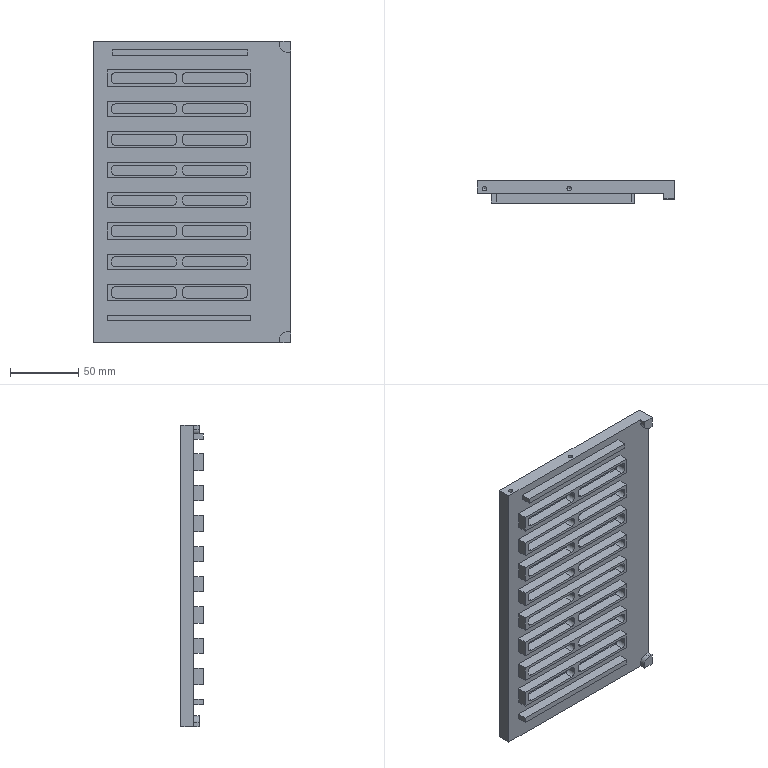NC program | NX | posted with a generic post | part box 144.5 x 16.5 x 221 mm
Lines 7394 to 8751 of 8751:
(FLOOR_WALL_1 , TOOL : D12-36-D12-120-3T-FINISH)
N14774 T20 M6
N14776 G53
N14778 G17 G0 G90 X1.505 Y-3.04 B0. C0. S4000 M3
N14780 G43 Z20. H20
N14782 Z-3.5
N14784 G94 G1 X2.265 Y-2.658 Z-3.545 F1000.
N14786 X6.037 Y-1.044 Z-3.76
N14788 X7.907 Y-0.376 Z-3.864
N14790 X6.484 Y0.28 Z-3.946
N14792 X3.712 Y1.744 Z-4.11
N14794 X2.368 Y2.55 Z-4.192
N14796 X-2.368 Z-4.44
N14798 X-3.962 Y1.594 Z-4.538
N14800 X-6.218 Y0.402 Z-4.672
N14802 X-7.907 Y-0.376 Z-4.769
N14804 X-6.037 Y-1.044 Z-4.873
N14806 X-2.265 Y-2.658 Z-5.088
N14808 X-0.491 Y-3.55 Z-5.192
N14810 X0.491 Z-5.244
N14812 X2.265 Y-2.658 Z-5.348
N14814 X6.037 Y-1.044 Z-5.563
N14816 X7.907 Y-0.376 Z-5.667
N14818 X6.484 Y0.28 Z-5.749
N14820 X3.712 Y1.744 Z-5.913
N14822 X2.368 Y2.55 Z-5.995
N14824 X-2.368 Z-6.244
N14826 X-3.962 Y1.594 Z-6.341
N14828 X-6.218 Y0.402 Z-6.475
N14830 X-7.907 Y-0.376 Z-6.572
N14832 X-6.037 Y-1.044 Z-6.676
N14834 X-2.265 Y-2.658 Z-6.891
N14836 X-0.491 Y-3.55 Z-6.995
N14838 X0.491 Z-7.047
N14840 X2.265 Y-2.658 Z-7.151
N14842 X6.037 Y-1.044 Z-7.366
N14844 X7.907 Y-0.376 Z-7.47
N14846 G2 X2.368 Y2.55 R57.6
N14848 G1 X-2.368
N14850 G2 X-7.907 Y-0.376 R57.6
N14852 G1 X-15.608 Y-0.596
N14854 X-7.907 Y-0.376
N14856 G2 X-0.491 Y-3.55 R65.7
N14858 G1 X0.491
N14860 G2 X7.907 Y-0.376 R65.7
N14862 G1 X15.608 Y-0.596
N14864 X7.907 Y-0.376
N14866 X29.55 Y4.006
N14868 G2 X5.158 Y12.15 R48.
N14870 G1 X-5.158
N14872 G2 X-43.194 Y5.267 R48.
N14874 G1 X-46.984 Y10.041
N14876 X-43.194 Y5.267
N14878 G2 X-44.576 Y-6.487 R48.
N14880 G1 X-49.193 Y-11.142
N14882 X-44.576 Y-6.487
N14884 G2 X-15.485 Y-8.06 R48.
N14886 X-2.863 Y-13.15 R56.1
N14888 G1 X2.863
N14890 G2 X15.485 Y-8.06 R56.1
N14892 X44.576 Y-6.487 R48.
N14894 G1 X49.193 Y-11.142
N14896 X44.576 Y-6.487
N14898 G2 X43.194 Y5.267 R48.
N14900 G1 X46.984 Y10.041
N14902 X43.194 Y5.267
N14904 G2 X29.55 Y4.006 R48.
N14906 G1 X8.274 Y21.75
N14908 X-8.274
N14910 G2 X-55.726 Y21.75 R38.4
N14912 G1 X-56.253
N14914 X-61.301 Y25.217
N14916 X-56.253 Y21.75
N14918 G2 X-55.46 Y19.009 R46.5
N14920 X-55.46 Y-9.109 R38.4
N14922 X-61. Y-22.086 R46.5
N14924 G1 Y-22.75
N14926 X-59.536
N14928 G2 X-46.559 Y-17.21 R46.5
N14930 X-18.441 Y-17.21 R38.4
N14932 X-5.464 Y-22.75 R46.5
N14934 G1 X5.464
N14936 G2 X18.441 Y-17.21 R46.5
N14938 X46.559 Y-17.21 R38.4
N14940 X59.536 Y-22.75 R46.5
N14942 G1 X61.
N14944 Y-22.086
N14946 G2 X55.46 Y-9.109 R46.5
N14948 X55.46 Y19.009 R38.4
N14950 X56.253 Y21.75 R46.5
N14952 G1 X61.301 Y25.217
N14954 X56.253 Y21.75
N14956 X55.726
N14958 G2 X8.274 Y21.75 R38.4
N14960 G1 X48.124 Y28.08
N14962 G2 X13.148 Y30.171 R28.8
N14964 X10.953 Y31.35 R36.9
N14966 G1 X-10.953
N14968 G2 X-13.148 Y30.171 R36.9
N14970 X-50.852 Y30.171 R28.8
N14972 X-53.047 Y31.35 R36.9
N14974 G1 X-70.6
N14976 Y29.074
N14978 G2 X-64.613 Y16.038 R36.9
N14980 X-64.613 Y-6.138 R28.8
N14982 X-70.6 Y-19.174 R36.9
N14984 G1 Y-32.35
N14986 X-56.624
N14988 G2 X-43.588 Y-26.363 R36.9
N14990 X-21.412 Y-26.363 R28.8
N14992 X-8.376 Y-32.35 R36.9
N14994 G1 X8.376
N14996 G2 X21.412 Y-26.363 R36.9
N14998 X43.588 Y-26.363 R28.8
N15000 X56.624 Y-32.35 R36.9
N15002 G1 X70.6
N15004 Y-19.174
N15006 G2 X64.613 Y-6.138 R36.9
N15008 X64.613 Y16.038 R28.8
N15010 X70.6 Y29.074 R36.9
N15012 G1 Y31.35
N15014 X53.047
N15016 G2 X50.852 Y30.171 R36.9
N15018 X48.124 Y28.08 R28.8
N15020 G1 X45.451 Y38.243
N15022 G2 X18.549 Y38.243 R19.2
N15024 X13.752 Y40.95 R27.3
N15026 G1 X-13.752
N15028 G2 X-18.549 Y38.243 R27.3
N15030 X-45.451 Y38.243 R19.2
N15032 X-50.248 Y40.95 R27.3
N15034 G1 X-77.252
N15036 G2 X-80.2 Y39.137 R27.3
N15038 G1 Y25.704
N15040 G2 X-73.776 Y13.03 R27.3
N15042 X-73.776 Y-3.13 R19.2
N15044 X-80.2 Y-15.804 R27.3
N15046 G1 Y-41.131
N15048 G2 X-79.246 Y-41.95 R27.3
N15050 G1 X-53.254
N15052 G2 X-40.58 Y-35.526 R27.3
N15054 X-24.42 Y-35.526 R19.2
N15056 X-11.746 Y-41.95 R27.3
N15058 G1 X11.746
N15060 G2 X24.42 Y-35.526 R27.3
N15062 X40.58 Y-35.526 R19.2
N15064 X53.254 Y-41.95 R27.3
N15066 G1 X79.246
N15068 G2 X80.2 Y-41.131 R27.3
N15070 G1 Y-15.804
N15072 G2 X73.776 Y-3.13 R27.3
N15074 X73.776 Y13.03 R19.2
N15076 X80.2 Y25.704 R27.3
N15078 G1 Y39.137
N15080 G2 X77.252 Y40.95 R27.3
N15082 G1 X50.248
N15084 G2 X45.451 Y38.243 R27.3
N15086 G1 X38.665 Y45.034
N15088 G2 X24.186 Y46.367 R9.6
N15090 X17.171 Y50.55 R17.7
N15092 G1 X-17.171
N15094 G2 X-24.186 Y46.367 R17.7
N15096 X-39.814 Y46.367 R9.6
N15098 X-46.829 Y50.55 R17.7
N15100 G1 X-80.671
N15102 G2 X-89.8 Y45.842 R17.7
N15104 G1 Y21.55
N15106 G2 X-82.971 Y9.905 R17.7
N15108 X-82.971 Y-0.005 R9.6
N15110 X-89.8 Y-11.65 R17.7
N15112 G1 Y-46.313
N15114 G2 X-83.4 Y-51.55 R17.7
N15116 G1 X-49.1
N15118 G2 X-37.455 Y-44.721 R17.7
N15120 X-27.545 Y-44.721 R9.6
N15122 X-15.9 Y-51.55 R17.7
N15124 G1 X15.9
N15126 G2 X27.545 Y-44.721 R17.7
N15128 X37.455 Y-44.721 R9.6
N15130 X49.1 Y-51.55 R17.7
N15132 G1 X83.4
N15134 G2 X89.8 Y-46.313 R17.7
N15136 G1 Y-11.65
N15138 G2 X82.971 Y-0.005 R17.7
N15140 X82.971 Y9.905 R9.6
N15142 X89.8 Y21.55 R17.7
N15144 G1 Y45.842
N15146 G2 X80.671 Y50.55 R17.7
N15148 G1 X46.829
N15150 G2 X39.814 Y46.367 R17.7
N15152 X38.665 Y45.034 R9.6
N15154 G1 X32. Y51.943
N15156 X29.873 Y55.15
N15158 X29.5
N15160 G2 X22.017 Y60.15 R8.1
N15162 G1 X-22.017
N15164 G2 X-29.5 Y55.15 R8.1
N15166 G1 X-29.873
N15168 X-32. Y51.943
N15170 X-34.127 Y55.15
N15172 X-34.5
N15174 G2 X-41.983 Y60.15 R8.1
N15176 G1 X-85.517
N15178 G2 X-93. Y55.15 R8.1
N15180 G1 X-99.4
N15182 Y15.475
N15184 G2 X-92.4 Y7.45 R8.1
N15186 G1 Y5.75
N15188 X-91.193 Y4.95
N15190 X-92.4 Y4.15
N15192 Y2.45
N15194 G2 X-99.4 Y-5.575 R8.1
N15196 G1 Y-54.15
N15198 X-97.5
N15200 G2 X-89.475 Y-61.15 R8.1
N15202 G1 X-43.025
N15204 G2 X-35. Y-54.15 R8.1
N15206 G1 X-33.3
N15208 X-32.5 Y-52.943
N15210 X-31.7 Y-54.15
N15212 X-30.
N15214 G2 X-21.975 Y-61.15 R8.1
N15216 G1 X21.975
N15218 G2 X30. Y-54.15 R8.1
N15220 G1 X31.7
N15222 X32.5 Y-52.943
N15224 X33.3 Y-54.15
N15226 X35.
N15228 G2 X43.025 Y-61.15 R8.1
N15230 G1 X89.475
N15232 G2 X97.5 Y-54.15 R8.1
N15234 G1 X99.4
N15236 Y-5.575
N15238 G2 X92.4 Y2.45 R8.1
N15240 G1 Y4.15
N15242 X91.193 Y4.95
N15244 X92.4 Y5.75
N15246 Y7.45
N15248 G2 X99.4 Y15.475 R8.1
N15250 G1 Y55.15
N15252 X93.
N15254 G2 X85.517 Y60.15 R8.1
N15256 G1 X41.983
N15258 G2 X34.5 Y55.15 R8.1
N15260 G1 X34.127
N15262 X32. Y51.943
N15264 X31.447 Y52.777
N15266 G2 X31.868 Y54.856 R1.5
N15268 G1 Z-4.47
N15270 G0 Z20.
N15272 M5
(PLANAR_MILL , TOOL : D8-25-D8-60-3T-FINISH)
N15274 T04 M6
N15276 G53
N15278 G17 G0 G90 X-119.5 Y76.35 B0. C0. S4000 M3
N15280 G43 Z20. H4
N15282 Z-13.
N15284 G94 G1 Z-15. F1000.
N15286 X-110.5
N15288 X110.5
N15290 X119.5
N15292 Z-13.
N15294 G0 Z20.
N15296 Y-76.35
N15298 Z-13.
N15300 G1 Z-15.
N15302 X110.5
N15304 X-110.5
N15306 X-119.5
N15308 Z-13.
N15310 G0 Z20.
(PLANAR_MILL_COPY , TOOL : D8-25-D8-60-3T-FINISH)
N15312 X-114.53 Y-81.25
N15314 Z-13.
N15316 G1 Z-15.
N15318 Y-72.25
N15320 Y72.25
N15322 Y81.25
N15324 Z-13.
N15326 G0 Z20.
N15328 X114.53
N15330 Z-13.
N15332 G1 Z-15.
N15334 Y72.25
N15336 Y-72.25
N15338 Y-81.25
N15340 Z-13.
N15342 G0 Z20.
N15344 M5
(FLOOR_WALL_1_COPY , TOOL : D5-15-D6-50-3T-FINISH)
N15346 T05 M6
N15348 G53
N15350 G17 G0 G90 X0.301 Y-1.523 B0. C0. S4000 M3
N15352 G43 Z20. H5
N15354 Z-6.5
N15356 G94 G1 X1.849 Y-0.757 Z-6.59 F1000.
N15358 X2.741 Y-0.357 Z-6.642
N15360 X4.608 Y0.4 Z-6.747
N15362 X4.296 Y0.523 Z-6.765
N15364 X3.985 Y0.65 Z-6.782
N15366 X-3.985 Z-7.2
N15368 X-4.296 Y0.523 Z-7.218
N15370 X-4.608 Y0.4 Z-7.235
N15372 X-2.741 Y-0.357 Z-7.341
N15374 X-1.849 Y-0.757 Z-7.392
N15376 X-0.043 Y-1.65 Z-7.498
N15378 X0. Z-7.5
N15380 X0.043
N15382 G2 X4.608 Y0.4 R67.6
N15384 G1 X7.216 Y0.41
N15386 X4.608 Y0.4
N15388 G2 X3.985 Y0.65 R67.6
N15390 G1 X-3.985
N15392 G2 X-4.608 Y0.4 R67.6
N15394 G1 X-7.216 Y0.41
N15396 X-4.608 Y0.4
N15398 G2 X-0.043 Y-1.65 R67.6
N15400 G1 X0.
N15402 Y-5.15
N15404 X0.873
N15406 G2 X16.666 Y0.448 R64.1
N15408 G1 X19.102 Y1.013
N15410 G3 X23.118 Y0.474 R63.1
N15412 X19.106 Y-0.097 R63.1
N15414 X19.102 Y1.013 R2.5
N15416 G1 X16.666 Y0.448
N15418 G2 X4.681 Y4.15 R64.1
N15420 G1 X-4.681
N15422 G2 X-16.666 Y0.448 R64.1
N15424 G1 X-19.106 Y-0.097
N15426 G3 X-23.118 Y0.474 R63.1
N15428 X-19.102 Y1.013 R63.1
N15430 X-19.106 Y-0.097 R2.5
N15432 G1 X-16.666 Y0.448
N15434 G2 X-0.873 Y-5.15 R64.1
N15436 G1 X0.
N15438 Y-8.65
N15440 X1.726
N15442 G2 X30. Y-1.65 R60.6
N15444 G1 X35.
N15446 G2 X40.054 Y-1.861 R60.6
N15448 X39.9 Y2.45 R60.6
N15450 G1 Y2.891
N15452 G2 X34.5 Y2.65 R60.6
N15454 G1 X29.5
N15456 G2 X5.396 Y7.65 R60.6
N15458 G1 X-5.396
N15460 G2 X-29.5 Y2.65 R60.6
N15462 G1 X-34.5
N15464 G2 X-39.9 Y2.891 R60.6
N15466 G1 Y2.45
N15468 G2 X-40.054 Y-1.861 R60.6
N15470 X-35. Y-1.65 R60.6
N15472 G1 X-30.
N15474 G2 X-1.726 Y-8.65 R60.6
N15476 G1 X0.
N15478 Y-12.15
N15480 X2.607
N15482 G2 X30. Y-5.15 R57.1
N15484 G1 X35.
N15486 G2 X44.009 Y-5.865 R57.1
N15488 X43.4 Y2.45 R57.1
N15490 G1 Y6.848
N15492 G2 X34.5 Y6.15 R57.1
N15494 G1 X29.5
N15496 G2 X6.133 Y11.15 R57.1
N15498 G1 X-6.133
N15500 G2 X-29.5 Y6.15 R57.1
N15502 G1 X-34.5
N15504 G2 X-43.4 Y6.848 R57.1
N15506 G1 Y2.45
N15508 G2 X-44.009 Y-5.865 R57.1
N15510 X-35. Y-5.15 R57.1
N15512 G1 X-30.
N15514 G2 X-2.607 Y-12.15 R57.1
N15516 G1 X0.
N15518 Y-15.65
N15520 X3.516
N15522 G2 X30. Y-8.65 R53.6
N15524 G1 X35.
N15526 G2 X48.455 Y-10.366 R53.6
N15528 X46.9 Y2.45 R53.6
N15530 G1 Y7.45
N15532 G2 X47.027 Y11.134 R53.6
N15534 X34.5 Y9.65 R53.6
N15536 G1 X29.5
N15538 G2 X6.895 Y14.65 R53.6
N15540 G1 X-6.895
N15542 G2 X-29.5 Y9.65 R53.6
N15544 G1 X-34.5
N15546 G2 X-47.027 Y11.134 R53.6
N15548 X-46.9 Y7.45 R53.6
N15550 G1 Y2.45
N15552 G2 X-48.455 Y-10.366 R53.6
N15554 X-35. Y-8.65 R53.6
N15556 G1 X-30.
N15558 G2 X-3.516 Y-15.65 R53.6
N15560 G1 X0.
N15562 Y-19.15
N15564 X4.458
N15566 G2 X30. Y-12.15 R50.1
N15568 G1 X35.
N15570 G2 X53.855 Y-15.834 R50.1
N15572 G1 X55.657 Y-17.657
N15574 X53.855 Y-15.834
N15576 G2 X50.4 Y2.45 R50.1
N15578 G1 Y7.45
N15580 G2 X51.134 Y15.992 R50.1
N15582 X34.5 Y13.15 R50.1
N15584 G1 X29.5
N15586 G2 X7.683 Y18.15 R50.1
N15588 G1 X-7.683
N15590 G2 X-29.5 Y13.15 R50.1
N15592 G1 X-34.5
N15594 G2 X-51.134 Y15.992 R50.1
N15596 X-50.4 Y7.45 R50.1
N15598 G1 Y2.45
N15600 G2 X-53.855 Y-15.834 R50.1
N15602 G1 X-55.657 Y-17.657
N15604 X-53.855 Y-15.834
N15606 G2 X-35. Y-12.15 R50.1
N15608 G1 X-30.
N15610 G2 X-4.458 Y-19.15 R50.1
N15612 G1 X0.
N15614 Y-22.65
N15616 X5.436
N15618 G2 X30. Y-15.65 R46.6
N15620 G1 X35.
N15622 G2 X59.564 Y-22.65 R46.6
N15624 G1 X60.9
N15626 Y-22.114
N15628 G2 X53.9 Y2.45 R46.6
N15630 G1 Y7.45
N15632 G2 X56.116 Y21.65 R46.6
N15634 G1 X55.5
N15636 G2 X34.5 Y16.65 R46.6
N15638 G1 X29.5
N15640 G2 X8.5 Y21.65 R46.6
N15642 G1 X-8.5
N15644 G2 X-29.5 Y16.65 R46.6
N15646 G1 X-34.5
N15648 G2 X-55.5 Y21.65 R46.6
N15650 G1 X-56.116
N15652 G2 X-53.9 Y7.45 R46.6
N15654 G1 Y2.45
N15656 G2 X-60.9 Y-22.114 R46.6
N15658 G1 Y-22.65
N15660 X-59.564
N15662 G2 X-35. Y-15.65 R46.6
N15664 G1 X-30.
N15666 G2 X-5.436 Y-22.65 R46.6
N15668 G1 X0.
N15670 Y-26.15
N15672 X6.454
N15674 G2 X30. Y-19.15 R43.1
N15676 G1 X35.
N15678 G2 X58.546 Y-26.15 R43.1
N15680 G1 X64.4
N15682 Y-21.096
N15684 G2 X57.4 Y2.45 R43.1
N15686 G1 Y7.45
N15688 G2 X61.202 Y25.15 R43.1
N15690 G1 X54.649
N15692 G2 X34.5 Y20.15 R43.1
N15694 G1 X29.5
N15696 G2 X9.351 Y25.15 R43.1
N15698 G1 X-9.351
N15700 G2 X-29.5 Y20.15 R43.1
N15702 G1 X-34.5
N15704 G2 X-54.649 Y25.15 R43.1
N15706 G1 X-61.202
N15708 G2 X-57.4 Y7.45 R43.1
N15710 G1 Y2.45
N15712 G2 X-64.4 Y-21.096 R43.1
N15714 G1 Y-26.15
N15716 X-58.546
N15718 G2 X-35. Y-19.15 R43.1
N15720 G1 X-30.
N15722 G2 X-6.454 Y-26.15 R43.1
N15724 G1 X0.
N15726 Y-29.65
N15728 X7.519
N15730 G2 X30. Y-22.65 R39.6
N15732 G1 X35.
N15734 G2 X57.481 Y-29.65 R39.6
N15736 G1 X67.9
N15738 Y-20.031
N15740 G2 X60.9 Y2.45 R39.6
N15742 G1 Y7.45
N15744 G2 X67.053 Y28.65 R39.6
N15746 G1 X53.761
N15748 G2 X34.5 Y23.65 R39.6
N15750 G1 X29.5
N15752 G2 X10.239 Y28.65 R39.6
N15754 G1 X-10.239
N15756 G2 X-29.5 Y23.65 R39.6
N15758 G1 X-34.5
N15760 G2 X-53.761 Y28.65 R39.6
N15762 G1 X-67.053
N15764 G2 X-60.9 Y7.45 R39.6
N15766 G1 Y2.45
N15768 G2 X-67.9 Y-20.031 R39.6
N15770 G1 Y-29.65
N15772 X-57.481
N15774 G2 X-35. Y-22.65 R39.6
N15776 G1 X-30.
N15778 G2 X-7.519 Y-29.65 R39.6
N15780 G1 X0.
N15782 Y-33.15
N15784 X8.636
N15786 G2 X30. Y-26.15 R36.1
N15788 G1 X35.
N15790 G2 X56.364 Y-33.15 R36.1
N15792 G1 X71.4
N15794 Y-18.914
N15796 G2 X64.4 Y2.45 R36.1
N15798 G1 Y7.45
N15800 G2 X71.4 Y28.814 R36.1
N15802 G1 Y32.15
N15804 X52.83
N15806 G2 X34.5 Y27.15 R36.1
N15808 G1 X29.5
N15810 G2 X11.17 Y32.15 R36.1
N15812 G1 X-11.17
N15814 G2 X-29.5 Y27.15 R36.1
N15816 G1 X-34.5
N15818 G2 X-52.83 Y32.15 R36.1
N15820 G1 X-71.4
N15822 Y28.814
N15824 G2 X-64.4 Y7.45 R36.1
N15826 G1 Y2.45
N15828 G2 X-71.4 Y-18.914 R36.1
N15830 G1 Y-33.15
N15832 X-56.364
N15834 G2 X-35. Y-26.15 R36.1
N15836 G1 X-30.
N15838 G2 X-8.636 Y-33.15 R36.1
N15840 G1 X0.
N15842 Y-36.65
N15844 X9.816
N15846 G2 X30. Y-29.65 R32.6
N15848 G1 X35.
N15850 G2 X55.184 Y-36.65 R32.6
N15852 G1 X74.9
N15854 Y-17.734
N15856 G2 X67.9 Y2.45 R32.6
N15858 G1 Y7.45
N15860 G2 X74.9 Y27.634 R32.6
N15862 G1 Y35.65
N15864 X51.849
N15866 G2 X34.5 Y30.65 R32.6
N15868 G1 X29.5
N15870 G2 X12.151 Y35.65 R32.6
N15872 G1 X-12.151
N15874 G2 X-29.5 Y30.65 R32.6
N15876 G1 X-34.5
N15878 G2 X-51.849 Y35.65 R32.6
N15880 G1 X-74.9
N15882 Y27.634
N15884 G2 X-67.9 Y7.45 R32.6
N15886 G1 Y2.45
N15888 G2 X-74.9 Y-17.734 R32.6
N15890 G1 Y-36.65
N15892 X-55.184
N15894 G2 X-35. Y-29.65 R32.6
N15896 G1 X-30.
N15898 G2 X-9.816 Y-36.65 R32.6
N15900 G1 X0.
N15902 Y-40.15
N15904 X11.069
N15906 G2 X30. Y-33.15 R29.1
N15908 G1 X35.
N15910 G2 X53.931 Y-40.15 R29.1
N15912 G1 X78.4
N15914 Y-16.481
N15916 G2 X71.4 Y2.45 R29.1
N15918 G1 Y7.45
N15920 G2 X78.4 Y26.381 R29.1
N15922 G1 Y38.078
N15924 G2 X76.69 Y39.15 R29.1
N15926 G1 X50.81
N15928 G2 X34.5 Y34.15 R29.1
N15930 G1 X29.5
N15932 G2 X13.19 Y39.15 R29.1
N15934 G1 X-13.19
N15936 G2 X-29.5 Y34.15 R29.1
N15938 G1 X-34.5
N15940 G2 X-50.81 Y39.15 R29.1
N15942 G1 X-76.69
N15944 G2 X-78.4 Y38.078 R29.1
N15946 G1 Y26.381
N15948 G2 X-71.4 Y7.45 R29.1
N15950 G1 Y2.45
N15952 G2 X-78.4 Y-16.481 R29.1
N15954 G1 Y-40.15
N15956 X-53.931
N15958 G2 X-35. Y-33.15 R29.1
N15960 G1 X-30.
N15962 G2 X-11.069 Y-40.15 R29.1
N15964 G1 X0.
N15966 Y-43.65
N15968 X12.41
N15970 G2 X30. Y-36.65 R25.6
N15972 G1 X35.
N15974 G2 X52.59 Y-43.65 R25.6
N15976 G1 X79.91
N15978 G2 X81.9 Y-41.952 R25.6
N15980 G1 Y-15.14
N15982 G2 X74.9 Y2.45 R25.6
N15984 G1 Y7.45
N15986 G2 X81.9 Y25.04 R25.6
N15988 G1 Y40.182
N15990 G2 X77.801 Y42.65 R25.6
N15992 G1 X49.699
N15994 G2 X34.5 Y37.65 R25.6
N15996 G1 X29.5
N15998 G2 X14.301 Y42.65 R25.6
N16000 G1 X-14.301
N16002 G2 X-29.5 Y37.65 R25.6
N16004 G1 X-34.5
N16006 G2 X-49.699 Y42.65 R25.6
N16008 G1 X-77.801
N16010 G2 X-81.9 Y40.182 R25.6
N16012 G1 Y25.04
N16014 G2 X-74.9 Y7.45 R25.6
N16016 G1 Y2.45
N16018 G2 X-81.9 Y-15.14 R25.6
N16020 G1 Y-41.952
N16022 G2 X-79.91 Y-43.65 R25.6
N16024 G1 X-52.59
N16026 G2 X-35. Y-36.65 R25.6
N16028 G1 X-30.
N16030 G2 X-12.41 Y-43.65 R25.6
N16032 G1 X0.
N16034 Y-47.15
N16036 X13.863
N16038 G2 X30. Y-40.15 R22.1
N16040 G1 X35.
N16042 G2 X51.137 Y-47.15 R22.1
N16044 G1 X81.363
N16046 G2 X85.4 Y-43.757 R22.1
N16048 G1 Y-13.687
N16050 G2 X78.4 Y2.45 R22.1
N16052 G1 Y7.45
N16054 G2 X85.4 Y23.587 R22.1
N16056 G1 Y42.498
N16058 G2 X79. Y46.15 R22.1
N16060 G1 X48.5
N16062 G2 X34.5 Y41.15 R22.1
N16064 G1 X29.5
N16066 G2 X15.5 Y46.15 R22.1
N16068 G1 X-15.5
N16070 G2 X-29.5 Y41.15 R22.1
N16072 G1 X-34.5
N16074 G2 X-48.5 Y46.15 R22.1
N16076 G1 X-79.
N16078 G2 X-85.4 Y42.498 R22.1
N16080 G1 Y23.587
N16082 G2 X-78.4 Y7.45 R22.1
N16084 G1 Y2.45
N16086 G2 X-85.4 Y-13.687 R22.1
N16088 G1 Y-43.757
N16090 G2 X-81.363 Y-47.15 R22.1
N16092 G1 X-51.137
N16094 G2 X-35. Y-40.15 R22.1
N16096 G1 X-30.
N16098 G2 X-13.863 Y-47.15 R22.1
N16100 G1 X0.
N16102 Y-50.65
N16104 X15.46
N16106 G2 X30. Y-43.65 R18.6
N16108 G1 X35.
N16110 G2 X49.54 Y-50.65 R18.6
N16112 G1 X82.96
N16114 G2 X88.9 Y-45.758 R18.6
N16116 G1 Y-12.09
N16118 G2 X81.9 Y2.45 R18.6
N16120 G1 Y7.45
N16122 G2 X88.9 Y21.99 R18.6
N16124 G1 Y45.108
N16126 G2 X80.311 Y49.65 R18.6
N16128 G1 X47.189
N16130 G2 X34.5 Y44.65 R18.6
N16132 G1 X29.5
N16134 G2 X16.811 Y49.65 R18.6
N16136 G1 X-16.811
N16138 G2 X-29.5 Y44.65 R18.6
N16140 G1 X-34.5
N16142 G2 X-47.189 Y49.65 R18.6
N16144 G1 X-80.311
N16146 G2 X-88.9 Y45.108 R18.6
N16148 G1 Y21.99
N16150 G2 X-81.9 Y7.45 R18.6
N16152 G1 Y2.45
N16154 G2 X-88.9 Y-12.09 R18.6
N16156 G1 Y-45.758
N16158 G2 X-82.96 Y-50.65 R18.6
N16160 G1 X-49.54
N16162 G2 X-35. Y-43.65 R18.6
N16164 G1 X-30.
N16166 G2 X-15.46 Y-50.65 R18.6
N16168 G1 X0.
N16170 Y-54.15
N16172 X17.256
N16174 G2 X30. Y-47.15 R15.1
N16176 G1 X35.
N16178 G2 X47.744 Y-54.15 R15.1
N16180 G1 X84.756
N16182 G2 X92.4 Y-48.037 R15.1
N16184 G1 Y-10.294
N16186 G2 X85.4 Y2.45 R15.1
N16188 G1 Y7.45
N16190 G2 X92.4 Y20.194 R15.1
N16192 G1 Y48.162
N16194 G2 X81.775 Y53.15 R15.1
N16196 G1 X45.725
N16198 G2 X34.5 Y48.15 R15.1
N16200 G1 X29.5
N16202 G2 X18.275 Y53.15 R15.1
N16204 G1 X-18.275
N16206 G2 X-29.5 Y48.15 R15.1
N16208 G1 X-34.5
N16210 G2 X-45.725 Y53.15 R15.1
N16212 G1 X-81.775
N16214 G2 X-92.4 Y48.162 R15.1
N16216 G1 Y20.194
N16218 G2 X-85.4 Y7.45 R15.1
N16220 G1 Y2.45
N16222 G2 X-92.4 Y-10.294 R15.1
N16224 G1 Y-48.037
N16226 G2 X-84.756 Y-54.15 R15.1
N16228 G1 X-47.744
N16230 G2 X-35. Y-47.15 R15.1
N16232 G1 X-30.
N16234 G2 X-17.256 Y-54.15 R15.1
N16236 G1 X0.
N16238 Y-57.65
N16240 X19.351
N16242 G2 X30. Y-50.65 R11.6
N16244 G1 X35.
N16246 G2 X45.649 Y-57.65 R11.6
N16248 G1 X86.851
N16250 G2 X95.9 Y-50.761 R11.6
N16252 G1 Y-8.199
N16254 G2 X88.9 Y2.45 R11.6
N16256 G1 Y7.45
N16258 G2 X95.9 Y18.099 R11.6
N16260 G1 Y51.65
N16262 X93.
N16264 G2 X83.461 Y56.65 R11.6
N16266 G1 X44.039
N16268 G2 X34.5 Y51.65 R11.6
N16270 G1 X29.5
N16272 G2 X19.961 Y56.65 R11.6
N16274 G1 X-19.961
N16276 G2 X-29.5 Y51.65 R11.6
N16278 G1 X-34.5
N16280 G2 X-44.039 Y56.65 R11.6
N16282 G1 X-83.461
N16284 G2 X-93. Y51.65 R11.6
N16286 G1 X-95.9
N16288 Y18.099
N16290 G2 X-88.9 Y7.45 R11.6
N16292 G1 Y2.45
N16294 G2 X-95.9 Y-8.199 R11.6
N16296 G1 Y-50.761
N16298 G2 X-86.851 Y-57.65 R11.6
N16300 G1 X-45.649
N16302 G2 X-35. Y-50.65 R11.6
N16304 G1 X-30.
N16306 G2 X-19.351 Y-57.65 R11.6
N16308 G1 X0.
N16310 Y-61.15
N16312 X21.975
N16314 G2 X30. Y-54.15 R8.1
N16316 G1 X35.
N16318 G2 X43.025 Y-61.15 R8.1
N16320 G1 X89.475
N16322 G2 X97.5 Y-54.15 R8.1
N16324 G1 X99.4
N16326 Y-5.575
N16328 G2 X92.4 Y2.45 R8.1
N16330 G1 Y7.45
N16332 G2 X99.4 Y15.475 R8.1
N16334 G1 Y55.15
N16336 X93.
N16338 G2 X85.517 Y60.15 R8.1
N16340 G1 X41.983
N16342 G2 X34.5 Y55.15 R8.1
N16344 G1 X29.5
N16346 G2 X22.017 Y60.15 R8.1
N16348 G1 X-22.017
N16350 G2 X-29.5 Y55.15 R8.1
N16352 G1 X-34.5
N16354 G2 X-41.983 Y60.15 R8.1
N16356 G1 X-85.517
N16358 G2 X-93. Y55.15 R8.1
N16360 G1 X-99.4
N16362 Y15.475
N16364 G2 X-92.4 Y7.45 R8.1
N16366 G1 Y2.45
N16368 G2 X-99.4 Y-5.575 R8.1
N16370 G1 Y-54.15
N16372 X-97.5
N16374 G2 X-89.475 Y-61.15 R8.1
N16376 G1 X-43.025
N16378 G2 X-35. Y-54.15 R8.1
N16380 G1 X-30.
N16382 G2 X-21.975 Y-61.15 R8.1
N16384 G1 X0.
N16386 Y-64.65
N16388 X24.975
N16390 G3 X25.387 Y-64.347 R0.42
N16392 G1 X25.4 Y-64.218
N16394 Y-62.25
N16396 G2 X30. Y-57.65 R4.6
N16398 G1 X35.
N16400 G2 X39.6 Y-62.25 R4.6
N16402 G1 X39.603 Y-64.291
N16404 G3 X40.032 Y-64.65 R0.418
N16406 G1 X92.475
N16408 X92.754 Y-64.558
N16410 X92.845 Y-64.505
N16412 X92.869 Y-64.402
N16414 X92.9 Y-64.218
N16416 Y-62.25
N16418 G2 X97.5 Y-57.65 R4.6
N16420 G1 X102.5
N16422 G3 X102.9 Y-57.25 R0.4
N16424 G1 Y-2.55
N16426 G3 X102.5 Y-2.15 R0.4
N16428 G1 X100.5
N16430 G2 X95.9 Y2.45 R4.6
N16432 G1 Y7.45
N16434 G2 X100.5 Y12.05 R4.6
N16436 G1 X102.5
N16438 G3 X102.9 Y12.45 R0.4
N16440 G1 Y58.25
N16442 G3 X102.5 Y58.65 R0.4
N16444 G1 X93.
N16446 G2 X88.4 Y63.25 R4.6
N16448 G3 X88. Y63.65 R0.4
N16450 G1 X39.5
N16452 G3 X39.1 Y63.25 R0.4
N16454 G2 X34.5 Y58.65 R4.6
N16456 G1 X29.5
N16458 G2 X24.9 Y63.25 R4.6
N16460 G3 X24.5 Y63.65 R0.4
N16462 G1 X-24.5
N16464 G3 X-24.9 Y63.25 R0.4
N16466 G2 X-29.5 Y58.65 R4.6
N16468 G1 X-34.5
N16470 G2 X-39.1 Y63.25 R4.6
N16472 G3 X-39.5 Y63.65 R0.4
N16474 G1 X-88.
N16476 G3 X-88.4 Y63.25 R0.4
N16478 G2 X-93. Y58.65 R4.6
N16480 G1 X-102.5
N16482 G3 X-102.9 Y58.25 R0.4
N16484 G1 Y12.45
N16486 G3 X-102.5 Y12.05 R0.4
N16488 G1 X-100.5
N16490 G2 X-95.9 Y7.45 R4.6
N16492 G1 Y2.45
N16494 G2 X-100.5 Y-2.15 R4.6
N16496 G1 X-102.5
N16498 G3 X-102.9 Y-2.55 R0.4
N16500 G1 Y-57.25
N16502 G3 X-102.5 Y-57.65 R0.4
N16504 G1 X-97.5
N16506 G2 X-92.9 Y-62.25 R4.6
N16508 G1 X-92.897 Y-64.291
N16510 G3 X-92.688 Y-64.602 R0.399
N16512 G1 X-92.468 Y-64.65
N16514 X-40.025
N16516 G3 X-39.631 Y-64.402 R0.42
N16518 G1 X-39.575 Y-64.317
N16520 X-39.6 Y-64.218
N16522 Y-62.25
N16524 G2 X-35. Y-57.65 R4.6
N16526 G1 X-30.
N16528 G2 X-25.4 Y-62.25 R4.6
N16530 G1 X-25.399 Y-64.271
N16532 X-25.391 Y-64.33
N16534 G3 X-24.968 Y-64.65 R0.419
N16536 G1 X0.
N16538 X1.
N16540 G3 X2.25 Y-63.4 R1.25
N16542 G1 Z-4.5
N16544 G0 Z20.
(PLANAR_MILL_1 , TOOL : D5-15-D6-50-3T-FINISH)
N16546 X-100.5 Y56.72 S3500
N16548 Z-5.48
N16550 G1 Z-7.48 F800.
N16552 G3 X-102.5 Y58.72 R2.
N16554 X-102.97 Y58.25 R0.47
N16556 G1 Y12.45
N16558 G3 X-102.5 Y11.98 R0.47
N16560 G1 X-100.5
N16562 G2 X-95.97 Y7.45 R4.53
N16564 G1 Y2.45
N16566 G2 X-100.5 Y-2.08 R4.53
N16568 G1 X-102.5
N16570 G3 X-102.97 Y-2.55 R0.47
N16572 G1 Y-57.25
N16574 G3 X-102.5 Y-57.72 R0.47
N16576 G1 X-97.5
N16578 G2 X-92.97 Y-62.25 R4.53
N16580 G1 Y-64.25
N16582 G3 X-92.5 Y-64.72 R0.47
N16584 G1 X-40.
N16586 G3 X-39.53 Y-64.25 R0.47
N16588 G1 Y-62.25
N16590 G2 X-35. Y-57.72 R4.53
N16592 G1 X-30.
N16594 G2 X-25.47 Y-62.25 R4.53
N16596 G1 Y-64.25
N16598 G3 X-25. Y-64.72 R0.47
N16600 G1 X25.
N16602 G3 X25.47 Y-64.25 R0.47
N16604 G1 Y-62.25
N16606 G2 X30. Y-57.72 R4.53
N16608 G1 X35.
N16610 G2 X39.53 Y-62.25 R4.53
N16612 G1 Y-64.25
N16614 G3 X40. Y-64.72 R0.47
N16616 G1 X92.5
N16618 G3 X92.97 Y-64.25 R0.47
N16620 G1 Y-62.25
N16622 G2 X97.5 Y-57.72 R4.53
N16624 G1 X102.5
N16626 G3 X102.97 Y-57.25 R0.47
N16628 G1 Y-2.55
N16630 G3 X102.5 Y-2.08 R0.47
N16632 G1 X100.5
N16634 G2 X95.97 Y2.45 R4.53
N16636 G1 Y7.45
N16638 G2 X100.5 Y11.98 R4.53
N16640 G1 X102.5
N16642 G3 X102.97 Y12.45 R0.47
N16644 G1 Y58.25
N16646 G3 X102.5 Y58.72 R0.47
N16648 G1 X93.
N16650 G2 X88.47 Y63.25 R4.53
N16652 G3 X88. Y63.72 R0.47
N16654 G1 X39.5
N16656 G3 X39.03 Y63.25 R0.47
N16658 G2 X34.5 Y58.72 R4.53
N16660 G1 X29.5
N16662 G2 X24.97 Y63.25 R4.53
N16664 G3 X24.5 Y63.72 R0.47
N16666 G1 X-24.5
N16668 G3 X-24.97 Y63.25 R0.47
N16670 G2 X-29.5 Y58.72 R4.53
N16672 G1 X-34.5
N16674 G2 X-39.03 Y63.25 R4.53
N16676 G3 X-39.5 Y63.72 R0.47
N16678 G1 X-88.
N16680 G3 X-88.47 Y63.25 R0.47
N16682 G2 X-93. Y58.72 R4.53
N16684 G1 X-102.5
N16686 G3 X-100.5 Y56.72 R2.
N16688 X-102.5 Y58.72 R2.
N16690 X-102.97 Y58.25 R0.47
N16692 G1 Y12.45
N16694 G3 X-102.5 Y11.98 R0.47
N16696 G1 X-100.5
N16698 G2 X-95.97 Y7.45 R4.53
N16700 G1 Y2.45
N16702 G2 X-100.5 Y-2.08 R4.53
N16704 G1 X-102.5
N16706 G3 X-102.97 Y-2.55 R0.47
N16708 G1 Y-57.25
N16710 G3 X-102.5 Y-57.72 R0.47
N16712 G1 X-97.5
N16714 G2 X-92.97 Y-62.25 R4.53
N16716 G1 Y-64.25
N16718 G3 X-92.5 Y-64.72 R0.47
N16720 G1 X-40.
N16722 G3 X-39.53 Y-64.25 R0.47
N16724 G1 Y-62.25
N16726 G2 X-35. Y-57.72 R4.53
N16728 G1 X-30.
N16730 G2 X-25.47 Y-62.25 R4.53
N16732 G1 Y-64.25
N16734 G3 X-25. Y-64.72 R0.47
N16736 G1 X25.
N16738 G3 X25.47 Y-64.25 R0.47
N16740 G1 Y-62.25
N16742 G2 X30. Y-57.72 R4.53
N16744 G1 X35.
N16746 G2 X39.53 Y-62.25 R4.53
N16748 G1 Y-64.25
N16750 G3 X40. Y-64.72 R0.47
N16752 G1 X92.5
N16754 G3 X92.97 Y-64.25 R0.47
N16756 G1 Y-62.25
N16758 G2 X97.5 Y-57.72 R4.53
N16760 G1 X102.5
N16762 G3 X102.97 Y-57.25 R0.47
N16764 G1 Y-2.55
N16766 G3 X102.5 Y-2.08 R0.47
N16768 G1 X100.5
N16770 G2 X95.97 Y2.45 R4.53
N16772 G1 Y7.45
N16774 G2 X100.5 Y11.98 R4.53
N16776 G1 X102.5
N16778 G3 X102.97 Y12.45 R0.47
N16780 G1 Y58.25
N16782 G3 X102.5 Y58.72 R0.47
N16784 G1 X93.
N16786 G2 X88.47 Y63.25 R4.53
N16788 G3 X88. Y63.72 R0.47
N16790 G1 X39.5
N16792 G3 X39.03 Y63.25 R0.47
N16794 G2 X34.5 Y58.72 R4.53
N16796 G1 X29.5
N16798 G2 X24.97 Y63.25 R4.53
N16800 G3 X24.5 Y63.72 R0.47
N16802 G1 X-24.5
N16804 G3 X-24.97 Y63.25 R0.47
N16806 G2 X-29.5 Y58.72 R4.53
N16808 G1 X-34.5
N16810 G2 X-39.03 Y63.25 R4.53
N16812 G3 X-39.5 Y63.72 R0.47
N16814 G1 X-88.
N16816 G3 X-88.47 Y63.25 R0.47
N16818 G2 X-93. Y58.72 R4.53
N16820 G1 X-102.5
N16822 G3 X-100.5 Y56.72 R2.
N16824 G1 Z-5.48
N16826 G0 Z20.
N16828 M5
(PLANAR_MILL_1_COPY , TOOL : 倒角D6-90度)
N16830 T06 M6
N16832 G53
N16834 G17 G0 G90 X-100.5 Y57.75 B0. C0. S3500 M3
N16836 G43 Z20. H6
N16838 Z0.5
N16840 G94 G1 Z-1.5 F1000.
N16842 G3 X-102.5 Y59.75 R2.
N16844 X-104. Y58.25 R1.5
N16846 G1 Y12.45
N16848 G3 X-102.5 Y10.95 R1.5
N16850 G1 X-100.5
N16852 G2 X-97. Y7.45 R3.5
N16854 G1 Y2.45
N16856 G2 X-100.5 Y-1.05 R3.5
N16858 G1 X-102.5
N16860 G3 X-104. Y-2.55 R1.5
N16862 G1 Y-57.25
N16864 G3 X-102.5 Y-58.75 R1.5
N16866 G1 X-97.5
N16868 G2 X-94. Y-62.25 R3.5
N16870 G1 Y-64.25
N16872 G3 X-92.5 Y-65.75 R1.5
N16874 G1 X-40.
N16876 G3 X-38.5 Y-64.25 R1.5
N16878 G1 Y-62.25
N16880 G2 X-35. Y-58.75 R3.5
N16882 G1 X-30.
N16884 G2 X-26.5 Y-62.25 R3.5
N16886 G1 Y-64.25
N16888 G3 X-25. Y-65.75 R1.5
N16890 G1 X25.
N16892 G3 X26.5 Y-64.25 R1.5
N16894 G1 Y-62.25
N16896 G2 X30. Y-58.75 R3.5
N16898 G1 X35.
N16900 G2 X38.5 Y-62.25 R3.5
N16902 G1 Y-64.25
N16904 G3 X40. Y-65.75 R1.5
N16906 G1 X92.5
N16908 G3 X94. Y-64.25 R1.5
N16910 G1 Y-62.25
N16912 G2 X97.5 Y-58.75 R3.5
N16914 G1 X102.5
N16916 G3 X104. Y-57.25 R1.5
N16918 G1 Y-2.55
N16920 G3 X102.5 Y-1.05 R1.5
N16922 G1 X100.5
N16924 G2 X97. Y2.45 R3.5
N16926 G1 Y7.45
N16928 G2 X100.5 Y10.95 R3.5
N16930 G1 X102.5
N16932 G3 X104. Y12.45 R1.5
N16934 G1 Y58.25
N16936 G3 X102.5 Y59.75 R1.5
N16938 G1 X93.
N16940 G2 X89.5 Y63.25 R3.5
N16942 G3 X88. Y64.75 R1.5
N16944 G1 X39.5
N16946 G3 X38. Y63.25 R1.5
N16948 G2 X34.5 Y59.75 R3.5
N16950 G1 X29.5
N16952 G2 X26. Y63.25 R3.5
N16954 G3 X24.5 Y64.75 R1.5
N16956 G1 X-24.5
N16958 G3 X-26. Y63.25 R1.5
N16960 G2 X-29.5 Y59.75 R3.5
N16962 G1 X-34.5
N16964 G2 X-38. Y63.25 R3.5
N16966 G3 X-39.5 Y64.75 R1.5
N16968 G1 X-88.
N16970 G3 X-89.5 Y63.25 R1.5
N16972 G2 X-93. Y59.75 R3.5
N16974 G1 X-102.5
N16976 G3 X-103.5 Y58.75 R1.
N16978 G1 X-102. Y57.75
N16980 Z0.5
N16982 G0 Z20.
N16984 M5
(PLANAR_MILL_1_COPY_COPY , TOOL : 刀杆C25-D25-150-2T)
N16986 T21 M6
N16988 G53
N16990 G17 G0 G90 X-83. Y-44.75 B0. C0. S3500 M3
N16992 G43 Z20. H21
N16994 Z2.
N16996 G94 G1 Z0. F800.
N16998 G3 X-108. Y-69.75 R25.
N17000 G1 X108.
N17002 Y69.75
N17004 X-108.
N17006 Y-69.75
N17008 G3 X-83. Y-44.75 R25.
N17010 G1 Z2.
N17012 G0 Z20.
N17014 M5
(ZLEVEL_PROFILE_STEEP , TOOL : D5-15-D6-50-3T-ROUGH)
N17016 T03 M6
N17018 G53
N17020 G17 G0 G90 X-9.5 Y-65.454 B0. C0. S4500 M3
N17022 G43 Z20. H3
N17024 Z0.97
N17026 G94 G1 Z-0.03 F2000.
N17028 Y-66.22
N17030 G3 X-8. Y-67.72 R1.5
N17032 G1 X8.
N17034 Y-67.69 Z-0.06
N17036 X-8.
N17038 Y-67.66 Z-0.09
N17040 X8.
N17042 Y-67.63 Z-0.12
N17044 X-8.
N17046 Y-67.6 Z-0.15
N17048 X8.
N17050 Y-67.57 Z-0.18
N17052 X-8.
N17054 Y-67.54 Z-0.21
N17056 X8.
N17058 Y-67.51 Z-0.24
N17060 X-8.
N17062 Y-67.48 Z-0.27
N17064 X8.
N17066 Y-67.45 Z-0.3
N17068 X-8.
N17070 Y-67.42 Z-0.33
N17072 X8.
N17074 Y-67.39 Z-0.36
N17076 X-8.
N17078 Y-67.36 Z-0.39
N17080 X8.
N17082 Y-67.33 Z-0.42
N17084 X-8.
N17086 Y-67.3 Z-0.45
N17088 X8.
N17090 Y-67.27 Z-0.48
N17092 X-8.
N17094 Y-67.24 Z-0.51
N17096 X8.
N17098 Y-67.21 Z-0.54
N17100 X-8.
N17102 Y-67.18 Z-0.57
N17104 X8.
N17106 Y-67.15 Z-0.6
N17108 X-8.
N17110 Y-67.12 Z-0.63
N17112 X8.
N17114 Y-67.09 Z-0.66
N17116 X-8.
N17118 Y-67.06 Z-0.69
N17120 X8.
N17122 Y-67.03 Z-0.72
N17124 X-8.
N17126 Y-67. Z-0.75
N17128 X8.
N17130 Y-66.97 Z-0.78
N17132 X-8.
N17134 Y-66.94 Z-0.81
N17136 X8.
N17138 Y-66.91 Z-0.84
N17140 X-8.
N17142 Y-66.88 Z-0.87
N17144 X8.
N17146 Y-66.85 Z-0.9
N17148 X-8.
N17150 Y-66.82 Z-0.93
N17152 X8.
N17154 Y-66.79 Z-0.96
N17156 X-8.
N17158 Y-66.76 Z-0.99
N17160 X8.
N17162 Y-66.73 Z-1.02
N17164 X-8.
N17166 Y-66.7 Z-1.05
N17168 X8.
N17170 Y-66.67 Z-1.08
N17172 X-8.
N17174 Y-66.64 Z-1.11
N17176 X8.
N17178 Y-66.61 Z-1.14
N17180 X-8.
N17182 Y-66.58 Z-1.17
N17184 X8.
N17186 Y-66.55 Z-1.2
N17188 X-8.
N17190 Y-66.52 Z-1.23
N17192 X8.
N17194 Y-66.49 Z-1.26
N17196 X-8.
N17198 Y-66.46 Z-1.29
N17200 X8.
N17202 Y-66.43 Z-1.32
N17204 X-8.
N17206 Y-66.4 Z-1.35
N17208 X8.
N17210 Y-66.37 Z-1.38
N17212 X-8.
N17214 Y-66.34 Z-1.41
N17216 X8.
N17218 Y-66.31 Z-1.44
N17220 X-8.
N17222 Y-66.28 Z-1.47
N17224 X8.
N17226 Y-66.25 Z-1.5
N17228 X-8.
N17230 Y-66.22 Z-1.53
N17232 X8.
N17234 Y-66.19 Z-1.56
N17236 X-8.
N17238 Y-66.16 Z-1.59
N17240 X8.
N17242 Y-66.13 Z-1.62
N17244 X-8.
N17246 Y-66.1 Z-1.65
N17248 X8.
N17250 Y-66.07 Z-1.68
N17252 X-8.
N17254 Y-66.04 Z-1.71
N17256 X8.
N17258 Y-66.01 Z-1.74
N17260 X-8.
N17262 Y-65.98 Z-1.77
N17264 X8.
N17266 Y-65.95 Z-1.8
N17268 X-8.
N17270 Y-65.92 Z-1.83
N17272 X8.
N17274 Y-65.89 Z-1.86
N17276 X-8.
N17278 Y-65.86 Z-1.89
N17280 X8.
N17282 Y-65.83 Z-1.92
N17284 X-8.
N17286 Y-65.8 Z-1.95
N17288 X8.
N17290 Y-65.77 Z-1.98
N17292 X-8.
N17294 Y-65.74 Z-2.01
N17296 X8.
N17298 Y-65.71 Z-2.04
N17300 X-8.
N17302 Y-65.68 Z-2.07
N17304 X8.
N17306 Y-65.65 Z-2.1
N17308 X-8.
N17310 Y-65.62 Z-2.13
N17312 X8.
N17314 Y-65.59 Z-2.16
N17316 X-8.
N17318 Y-65.56 Z-2.19
N17320 X8.
N17322 Y-65.53 Z-2.22
N17324 X-8.
N17326 Y-65.5 Z-2.25
N17328 X8.
N17330 Y-65.47 Z-2.28
N17332 X-8.
N17334 Y-65.44 Z-2.31
N17336 X8.
N17338 Y-65.41 Z-2.34
N17340 X-8.
N17342 Y-65.38 Z-2.37
N17344 X8.
N17346 Y-65.35 Z-2.4
N17348 X-8.
N17350 Y-65.32 Z-2.43
N17352 X8.
N17354 Y-65.29 Z-2.46
N17356 X-8.
N17358 Y-65.26 Z-2.49
N17360 X8.
N17362 Y-65.23 Z-2.52
N17364 X-8.
N17366 Y-65.2 Z-2.55
N17368 X8.
N17370 Y-65.17 Z-2.58
N17372 X-8.
N17374 Y-65.14 Z-2.61
N17376 X8.
N17378 Y-65.11 Z-2.64
N17380 X-8.
N17382 Y-65.08 Z-2.67
N17384 X8.
N17386 Y-65.05 Z-2.7
N17388 X-8.
N17390 Y-65.02 Z-2.73
N17392 X8.
N17394 Y-64.99 Z-2.76
N17396 X-8.
N17398 Y-64.96 Z-2.79
N17400 X8.
N17402 Y-64.93 Z-2.82
N17404 X-8.
N17406 Y-64.9 Z-2.85
N17408 X8.
N17410 Y-64.87 Z-2.88
N17412 X-8.
N17414 Y-64.84 Z-2.91
N17416 X8.
N17418 Y-64.81 Z-2.94
N17420 X-8.
N17422 Y-64.78 Z-2.97
N17424 X8.
N17426 Y-64.75 Z-3.
N17428 X-8.
N17430 G2 X-9.5 Y-63.25 R1.5
N17432 G1 Y-62.476
N17434 Z-2.
N17436 G0 Z20.
N17438 M5
N17440 M2